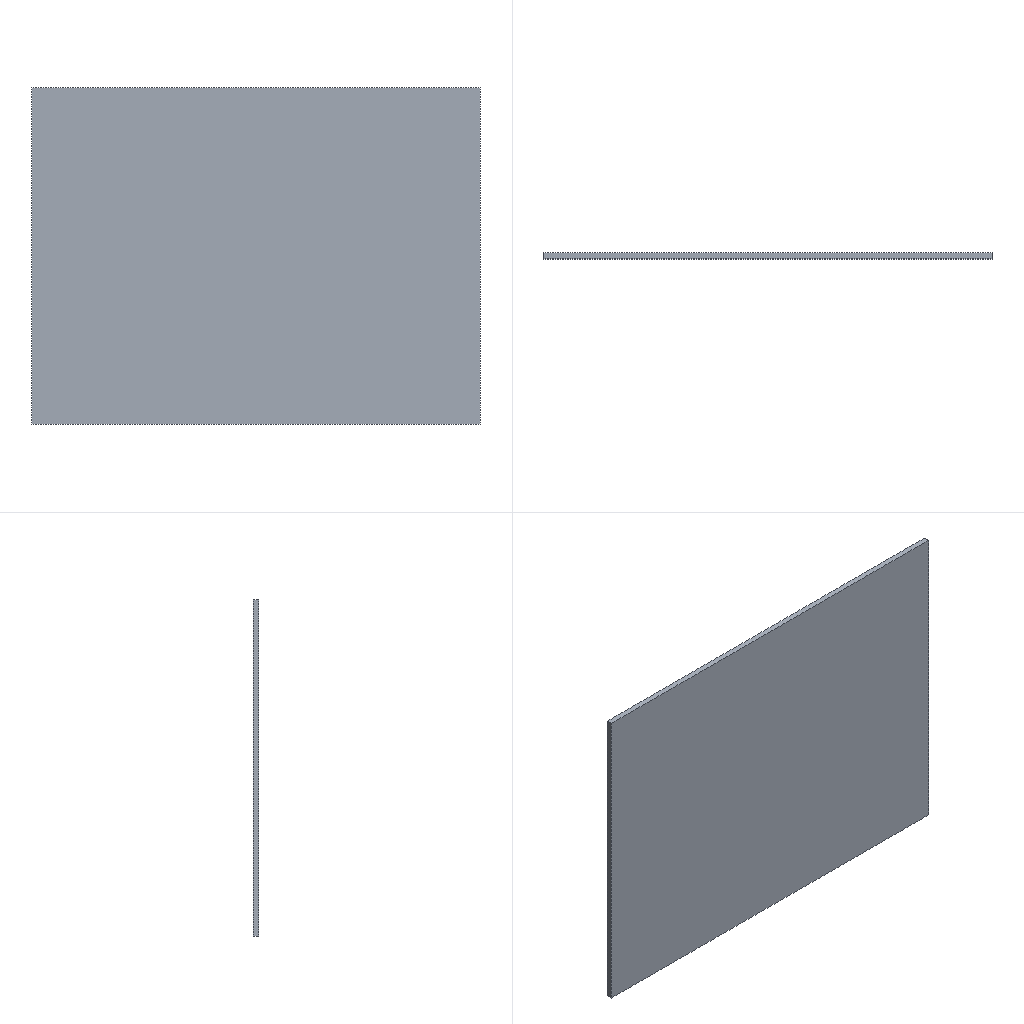Simulation study | ansys workbench
Ansys APDL input file, long lists of numbers shortened:
/batch
/config,noeldb,1     ! force off writing results to database
*get,_wallstrt,active,,time,wall
! ANSYS input file written by Workbench version 2022 R1
! File used for geometry attach: F:\ansys（分析文件汇总)\122\零件1.STEP
/title,wbnew--____ (B5)
! ****** Begin Custom Load Command Snippet ******
/COM, ACT Extensions:
/COM,     LSDYNA, 2021.1
/COM,
! ****** End   Custom Load Command Snippet ******
*DIM,_wb_ProjectScratch_dir,string,248
_wb_ProjectScratch_dir(1) = 'C:\Users\Administrator\AppData\Local\Temp\WB_Administrator_2068_2\_ProjectScratch\ScrDF2D\'
*DIM,_wb_SolverFiles_dir,string,248
_wb_SolverFiles_dir(1) = 'C:\Users\Administrator\AppData\Local\Temp\WB_Administrator_2068_2\wbnew_files\dp0\SYS\MECH\'
*DIM,_wb_userfiles_dir,string,248
_wb_userfiles_dir(1) = 'C:\Users\Administrator\AppData\Local\Temp\WB_Administrator_2068_2\wbnew_files\user_files\'
/com,--- Data in consistent NMM units. See Solving Units in the help system for more information.
/units,MPA
/nopr
/wb,file,start              !  signify a WB generated input file
/prep7
! Turn off shape checking because checks already performed inside WB mesher.
! See help system for more information.
SHPP,OFF,,NOWARN
/nolist
etcon,set             ! allow ANSYS to choose best KEYOP's for 180x elements, resets any applicable keyopt to MAPDL defaults
/com,*********** Nodes for the whole assembly ***********
nblock,3,,8485
(1i9,3e20.9e3)
        1     3.871770788E+01    -5.929089418E+00     0.000000000E+00
! (7713 more lines like these left out)
-1
/wb,elem,start            !  set before creation of elements
/com,*********** Elements for Body 1 "__1-FreeParts|__-__1" ***********
et,1,186
keyo,1,2,1          ! set full integration on SOLID186
eblock,19,solid,,1028
(19i9)
        1        1        1        1        0        0        0        0       20        0        1        4      850      851      811     1845      999      998     1038
! (2055 more lines like these left out)
-1
/wb,elem,end               !  done creating elements
/com,*********** Send User Defined Coordinate System(s) ***********
csys,0
toffst,273.15,  ! Temperature offset from absolute zero
/com,*********** Set Reference Temperature ***********
tref,22.
/wb,mat,start              !  starting to send materials
/com,*********** Send Materials ***********
Temperature = 'TEMP' ! Temperature
MP,DENS,1,7.85e-09,	! tonne mm^-3
MP,ALPX,1,1.2e-05,	! C^-1
MP,C,1,434000000,	! mm^2 s^-2 C^-1
MP,KXX,1,60.5,	! tonne mm s^-3 C^-1
MP,RSVX,1,0.00017,	! ohm mm
MP,EX,1,200000,	! tonne s^-2 mm^-1
MP,NUXY,1,0.3,
MP,MURX,1,10000,
/wb,mat,end                !  done sending materials
!************************* Model Summary ********************
!__1-FreeParts|__-__1,	结构钢,	matid,	1
!************************* End Model Summary ********************
! get the diagonal of the bounding box. Needed later for other things
*get,_xmin,node,,mnloc,x
*get,_ymin,node,,mnloc,y
*get,_zmin,node,,mnloc,z
*get,_xmax,node,,mxloc,x
*get,_ymax,node,,mxloc,y
*get,_zmax,node,,mxloc,z
_ASMDIAG=(_xmax-_xmin)*(_xmax-_xmin)+(_ymax-_ymin)*(_ymax-_ymin)+(_zmax-_zmin)*(_zmax-_zmin)
_ASMDIAG=SQRT(_ASMDIAG)
/wb,contact,start          !  starting to send contact
/wb,contact,end            !  done creating contacts
/golist
/wb,load,start             !  starting to send loads
/com,******* Constant Zero Displacement X *******
CMBLOCK,_DISPZEROUX,NODE,       78
(8i10)
      2041      2042      2043      2044      2045      2046      2047      2048
! (9 more lines like these left out)
cmsel,s,_DISPZEROUX
d,all,ux,0
nsel,all
/com,******* Constant Zero Displacement Y *******
CMBLOCK,_DISPZEROUY,NODE,       78
(8i10)
      2041      2042      2043      2044      2045      2046      2047      2048
! (9 more lines like these left out)
cmsel,s,_DISPZEROUY
d,all,uy,0
nsel,all
/com,******* Constant Zero Displacement Z *******
CMBLOCK,_DISPZEROUZ,NODE,       78
(8i10)
      2041      2042      2043      2044      2045      2046      2047      2048
! (9 more lines like these left out)
cmsel,s,_DISPZEROUZ
d,all,uz,0
nsel,all
/com,*********** Define Force Using Surface Effect Elements ***********
local,12,0,0.,0.,0.,0.,0.,0.
csys,0
et,2,154
eblock,10,,,15
(15i9)
     3293        2        2        2       12     2162     1951     1952     2161     7297     7296     7299     7612
! (14 more lines like these left out)
-1
esel,s,type,,2
keyop,2,2,1                ! Apply load in local coordinate system
keyop,2,7,1                ! Use original area so load is constant in large deformation
esel,all
/gst,on,on
fini
*get,_numnode,node,0,count
*get,_numelem,elem,0,count
*get, _MAXELEMNUM, elem, 0, NUM, MAX
*get, _MAXNODENUM, node, 0, NUM, MAX
*get, _MAXELEMTYPE, etyp, 0, NUM, MAX
*get, _MAXREALCONST, real, 0, NUM, MAX
/go
/wb,load,end               !  done creating loads
/com,--- Number of total nodes = %_numnode%
/com,--- Number of contact elements = 15
/com,--- Number of spring elements = 0
/com,--- Number of bearing elements = 0
/com,--- Number of solid elements = 1028
/com,--- Number of condensed parts = 0
/com,--- Number of total elements = %_numelem%
*get,_wallbsol,active,,time,wall
/com,****************************************************************************
/com,*************************    SOLUTION       ********************************
/com,****************************************************************************
/solu
antype,0                   ! static analysis
_thickRatio=  0     ! Ratio of thick parts in the model
eqsl,sparse,,,,,1
cntr,print,1               ! print out contact info and also make no initial contact an error
dmpoption,emat,no             ! Don't combine emat file for DANSYS
dmpoption,esav,no             ! Don't combine esav file for DANSYS
nldiag,cont,iter           ! print out contact info each equilibrium iteration
rescontrol,,none                 ! Do not keep any restart files
/com,****************************************************
/com,******************* SOLVE FOR LS 1 OF 1 ****************
esel,s,type,,2
nsle
sfe,all,1,pres,1,101.794
sfe,all,2,pres,1,0.
sfe,all,3,pres,1,0.
nsel,all
esel,all
/nopr
/gopr
nsub,1,1,1
time,1.
outres,erase
outres,all,none
outres,nsol,all,
outres,rsol,all
outres,eangl,all
outres,etmp,all
outres,veng,all
outres,strs,all,
outres,epel,all,
outres,eppl,all,
outres,cont,all,
! *********** WB SOLVE COMMAND ***********
! check interactive state
*get,ANSINTER_,active,,int
*if,ANSINTER_,ne,0,then
/eof
*endif
solve
/com *************** Write FE CONNECTORS *********
CEWRITE,file,ce,,INTE
/com,****************************************************
/com,*************** FINISHED SOLVE FOR LS 1 *************
*get,_wallasol,active,,time,wall
/nopr
*get,_numnode,node,0,count
*get,_numelem,elem,0,count
*get, _MAXELEMNUM, elem, 0, NUM, MAX
*get, _MAXNODENUM, node, 0, NUM, MAX,,,INTERNAL
*get, _MAXELEMTYPE, etyp, 0, NUM, MAX
*get, _MAXREALCONST, real, 0, NUM, MAX
/gopr
/post1
xmlo,ENCODING,ISO-8859-1
xmlo,parm
/xml,parm,xml
fini
/gopr
*get,_walldone,active,,time,wall
_preptime=(_wallbsol-_wallstrt)*3600
_solvtime=(_wallasol-_wallbsol)*3600
_posttime=(_walldone-_wallasol)*3600
_totaltim=(_walldone-_wallstrt)*3600
*get,_dlbratio,active,0,solu,dlbr
*get,_combtime,active,0,solu,comb
*get,_ssmode,active,0,solu,ssmm
*get,_ndofs,active,0,solu,ndof
*get,_sol_end_time,active,0,set,time
*if,_sol_end_time,eq,1.,then
/fclean				!clean distributed files
*endif
/com,--- Total number of nodes = %_numnode%
/com,--- Total number of elements = %_numelem%
/com,--- Element load balance ratio = %_dlbratio%
/com,--- Time to combine distributed files = %_combtime%
/com,--- Sparse memory mode = %_ssmode%
/com,--- Number of DOF = %_ndofs%
/wb,file,end               ! done with WB generated input